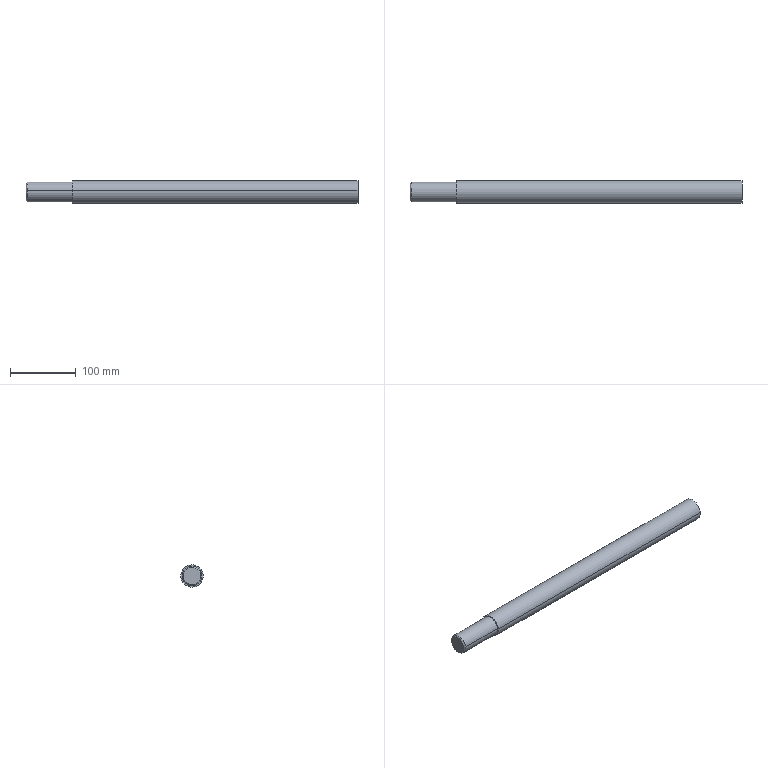Part | NX | features BREP 1 | 1 solid | 9 faces | box 504.795 x 33.982 x 33.982 mm | volume 443587 mm3 | cylinder 4 | plane 3 | cone 2 | commonest cylinder face diameters 30 x2 33.982 x2
STEP:
#1=CARTESIAN_POINT('',(560.635,-16.836,2.293));
#2=VERTEX_POINT('',#1);
#3=CARTESIAN_POINT('',(560.635,16.836,-2.293));
#4=VERTEX_POINT('',#3);
#5=CARTESIAN_POINT('',(560.635,0.,0.));
#6=DIRECTION('',(1.,0.,0.));
#7=DIRECTION('',(0.,0.,1.));
#8=AXIS2_PLACEMENT_3D('',#5,#6,#7);
#9=CIRCLE('',#8,16.991);
#10=EDGE_CURVE('',#2,#4,#9,.T.);
#11=ORIENTED_EDGE('',*,*,#10,.F.);
#12=CARTESIAN_POINT('',(126.35,-16.836,2.293));
#13=VERTEX_POINT('',#12);
#14=CARTESIAN_POINT('',(55.84,-16.836,2.293));
#15=DIRECTION('',(-1.,0.,0.));
#16=VECTOR('',#15,1000.);
#17=LINE('',#14,#16);
#18=EDGE_CURVE('',#2,#13,#17,.T.);
#19=ORIENTED_EDGE('',*,*,#18,.T.);
#20=CARTESIAN_POINT('',(126.35,16.836,-2.293));
#21=VERTEX_POINT('',#20);
#22=CARTESIAN_POINT('',(126.35,0.,0.));
#23=DIRECTION('',(1.,0.,0.));
#24=DIRECTION('',(0.,0.9909,-0.1349));
#25=AXIS2_PLACEMENT_3D('',#22,#23,#24);
#26=CIRCLE('',#25,16.991);
#27=EDGE_CURVE('',#13,#21,#26,.T.);
#28=ORIENTED_EDGE('',*,*,#27,.T.);
#29=CARTESIAN_POINT('',(55.84,16.836,-2.293));
#30=DIRECTION('',(-1.,0.,0.));
#31=VECTOR('',#30,1000.);
#32=LINE('',#29,#31);
#33=EDGE_CURVE('',#4,#21,#32,.T.);
#34=ORIENTED_EDGE('',*,*,#33,.F.);
#35=EDGE_LOOP('',(#11,#19,#28,#34));
#36=FACE_BOUND('',#35,.T.);
#37=CARTESIAN_POINT('',(55.84,0.,0.));
#38=DIRECTION('',(-1.,0.,0.));
#39=DIRECTION('',(0.,-0.9909,0.1349));
#40=AXIS2_PLACEMENT_3D('',#37,#38,#39);
#41=CYLINDRICAL_SURFACE('',#40,16.991);
#42=ADVANCED_FACE('',(#36),#41,.T.);
#43=CARTESIAN_POINT('',(126.35,14.863,-2.024));
#44=VERTEX_POINT('',#43);
#45=CARTESIAN_POINT('',(126.35,-14.863,2.024));
#46=VERTEX_POINT('',#45);
#47=CARTESIAN_POINT('',(126.35,0.,0.));
#48=DIRECTION('',(-1.,0.,0.));
#49=DIRECTION('',(0.,0.9909,-0.1349));
#50=AXIS2_PLACEMENT_3D('',#47,#48,#49);
#51=CIRCLE('',#50,15.);
#52=EDGE_CURVE('',#44,#46,#51,.T.);
#53=ORIENTED_EDGE('',*,*,#52,.T.);
#54=CARTESIAN_POINT('',(57.572,-14.863,2.024));
#55=VERTEX_POINT('',#54);
#56=CARTESIAN_POINT('',(55.84,-14.863,2.024));
#57=DIRECTION('',(-1.,0.,0.));
#58=VECTOR('',#57,1000.);
#59=LINE('',#56,#58);
#60=EDGE_CURVE('',#46,#55,#59,.T.);
#61=ORIENTED_EDGE('',*,*,#60,.T.);
#62=CARTESIAN_POINT('',(57.572,14.863,-2.024));
#63=VERTEX_POINT('',#62);
#64=CARTESIAN_POINT('',(57.572,0.,0.));
#65=DIRECTION('',(1.,0.,0.));
#66=DIRECTION('',(0.,0.9909,-0.1349));
#67=AXIS2_PLACEMENT_3D('',#64,#65,#66);
#68=CIRCLE('',#67,15.);
#69=EDGE_CURVE('',#55,#63,#68,.T.);
#70=ORIENTED_EDGE('',*,*,#69,.T.);
#71=CARTESIAN_POINT('',(55.84,14.863,-2.024));
#72=DIRECTION('',(-1.,0.,0.));
#73=VECTOR('',#72,1000.);
#74=LINE('',#71,#73);
#75=EDGE_CURVE('',#44,#63,#74,.T.);
#76=ORIENTED_EDGE('',*,*,#75,.F.);
#77=EDGE_LOOP('',(#53,#61,#70,#76));
#78=FACE_BOUND('',#77,.T.);
#79=CARTESIAN_POINT('',(55.84,0.,0.));
#80=DIRECTION('',(-1.,0.,0.));
#81=DIRECTION('',(0.,-0.9909,0.1349));
#82=AXIS2_PLACEMENT_3D('',#79,#80,#81);
#83=CYLINDRICAL_SURFACE('',#82,15.);
#84=ADVANCED_FACE('',(#78),#83,.T.);
#85=CARTESIAN_POINT('',(55.84,13.147,-1.79));
#86=VERTEX_POINT('',#85);
#87=CARTESIAN_POINT('',(55.84,-13.147,1.79));
#88=VERTEX_POINT('',#87);
#89=CARTESIAN_POINT('',(55.84,0.,0.));
#90=DIRECTION('',(-1.,0.,0.));
#91=DIRECTION('',(0.,0.9909,-0.1349));
#92=AXIS2_PLACEMENT_3D('',#89,#90,#91);
#93=CIRCLE('',#92,13.268);
#94=EDGE_CURVE('',#86,#88,#93,.T.);
#95=ORIENTED_EDGE('',*,*,#94,.F.);
#96=CARTESIAN_POINT('',(55.84,13.147,-1.79));
#97=DIRECTION('',(0.7071,0.7006,-0.09541));
#98=VECTOR('',#97,1000.);
#99=LINE('',#96,#98);
#100=EDGE_CURVE('',#63,#86,#99,.F.);
#101=ORIENTED_EDGE('',*,*,#100,.F.);
#102=ORIENTED_EDGE('',*,*,#69,.F.);
#103=CARTESIAN_POINT('',(55.84,-13.147,1.79));
#104=DIRECTION('',(0.7071,-0.7006,0.09541));
#105=VECTOR('',#104,1000.);
#106=LINE('',#103,#105);
#107=EDGE_CURVE('',#55,#88,#106,.F.);
#108=ORIENTED_EDGE('',*,*,#107,.T.);
#109=EDGE_LOOP('',(#95,#101,#102,#108));
#110=FACE_BOUND('',#109,.T.);
#111=CARTESIAN_POINT('',(55.84,0.,0.));
#112=DIRECTION('',(1.,0.,0.));
#113=DIRECTION('',(0.,0.9909,-0.1349));
#114=AXIS2_PLACEMENT_3D('',#111,#112,#113);
#115=CONICAL_SURFACE('',#114,13.268,0.7854);
#116=ADVANCED_FACE('',(#110),#115,.T.);
#117=CARTESIAN_POINT('',(55.84,0.,0.));
#118=DIRECTION('',(-1.,0.,0.));
#119=DIRECTION('',(0.,0.9909,-0.1349));
#120=AXIS2_PLACEMENT_3D('',#117,#118,#119);
#121=CIRCLE('',#120,13.268);
#122=EDGE_CURVE('',#88,#86,#121,.T.);
#123=ORIENTED_EDGE('',*,*,#122,.T.);
#124=ORIENTED_EDGE('',*,*,#94,.T.);
#125=EDGE_LOOP('',(#123,#124));
#126=FACE_BOUND('',#125,.T.);
#127=CARTESIAN_POINT('',(55.84,14.863,-2.024));
#128=DIRECTION('',(-1.,0.,0.));
#129=DIRECTION('',(0.,-0.9909,0.1349));
#130=AXIS2_PLACEMENT_3D('',#127,#128,#129);
#131=PLANE('',#130);
#132=ADVANCED_FACE('',(#126),#131,.T.);
#133=ORIENTED_EDGE('',*,*,#100,.T.);
#134=ORIENTED_EDGE('',*,*,#122,.F.);
#135=ORIENTED_EDGE('',*,*,#107,.F.);
#136=CARTESIAN_POINT('',(57.572,0.,0.));
#137=DIRECTION('',(1.,0.,0.));
#138=DIRECTION('',(0.,0.9909,-0.1349));
#139=AXIS2_PLACEMENT_3D('',#136,#137,#138);
#140=CIRCLE('',#139,15.);
#141=EDGE_CURVE('',#63,#55,#140,.T.);
#142=ORIENTED_EDGE('',*,*,#141,.F.);
#143=EDGE_LOOP('',(#133,#134,#135,#142));
#144=FACE_BOUND('',#143,.T.);
#145=CARTESIAN_POINT('',(55.84,0.,0.));
#146=DIRECTION('',(1.,0.,0.));
#147=DIRECTION('',(0.,0.9909,-0.1349));
#148=AXIS2_PLACEMENT_3D('',#145,#146,#147);
#149=CONICAL_SURFACE('',#148,13.268,0.7854);
#150=ADVANCED_FACE('',(#144),#149,.T.);
#151=ORIENTED_EDGE('',*,*,#60,.F.);
#152=CARTESIAN_POINT('',(126.35,0.,0.));
#153=DIRECTION('',(-1.,0.,0.));
#154=DIRECTION('',(0.,0.9909,-0.1349));
#155=AXIS2_PLACEMENT_3D('',#152,#153,#154);
#156=CIRCLE('',#155,15.);
#157=EDGE_CURVE('',#46,#44,#156,.T.);
#158=ORIENTED_EDGE('',*,*,#157,.T.);
#159=ORIENTED_EDGE('',*,*,#75,.T.);
#160=ORIENTED_EDGE('',*,*,#141,.T.);
#161=EDGE_LOOP('',(#151,#158,#159,#160));
#162=FACE_BOUND('',#161,.T.);
#163=CARTESIAN_POINT('',(55.84,0.,0.));
#164=DIRECTION('',(-1.,0.,0.));
#165=DIRECTION('',(0.,-0.9909,0.1349));
#166=AXIS2_PLACEMENT_3D('',#163,#164,#165);
#167=CYLINDRICAL_SURFACE('',#166,15.);
#168=ADVANCED_FACE('',(#162),#167,.T.);
#169=CARTESIAN_POINT('',(126.35,0.,0.));
#170=DIRECTION('',(1.,0.,0.));
#171=DIRECTION('',(0.,0.9909,-0.1349));
#172=AXIS2_PLACEMENT_3D('',#169,#170,#171);
#173=CIRCLE('',#172,16.991);
#174=EDGE_CURVE('',#21,#13,#173,.T.);
#175=ORIENTED_EDGE('',*,*,#174,.F.);
#176=ORIENTED_EDGE('',*,*,#27,.F.);
#177=EDGE_LOOP('',(#175,#176));
#178=FACE_BOUND('',#177,.T.);
#179=ORIENTED_EDGE('',*,*,#52,.F.);
#180=ORIENTED_EDGE('',*,*,#157,.F.);
#181=EDGE_LOOP('',(#179,#180));
#182=FACE_BOUND('',#181,.T.);
#183=CARTESIAN_POINT('',(126.35,16.836,-2.293));
#184=DIRECTION('',(-1.,0.,0.));
#185=DIRECTION('',(0.,-0.9909,0.1349));
#186=AXIS2_PLACEMENT_3D('',#183,#184,#185);
#187=PLANE('',#186);
#188=ADVANCED_FACE('',(#178,#182),#187,.T.);
#189=ORIENTED_EDGE('',*,*,#18,.F.);
#190=CARTESIAN_POINT('',(560.635,0.,0.));
#191=DIRECTION('',(1.,0.,0.));
#192=DIRECTION('',(0.,0.,1.));
#193=AXIS2_PLACEMENT_3D('',#190,#191,#192);
#194=CIRCLE('',#193,16.991);
#195=EDGE_CURVE('',#4,#2,#194,.T.);
#196=ORIENTED_EDGE('',*,*,#195,.F.);
#197=ORIENTED_EDGE('',*,*,#33,.T.);
#198=ORIENTED_EDGE('',*,*,#174,.T.);
#199=EDGE_LOOP('',(#189,#196,#197,#198));
#200=FACE_BOUND('',#199,.T.);
#201=CARTESIAN_POINT('',(55.84,0.,0.));
#202=DIRECTION('',(-1.,0.,0.));
#203=DIRECTION('',(0.,-0.9909,0.1349));
#204=AXIS2_PLACEMENT_3D('',#201,#202,#203);
#205=CYLINDRICAL_SURFACE('',#204,16.991);
#206=ADVANCED_FACE('',(#200),#205,.T.);
#207=ORIENTED_EDGE('',*,*,#195,.T.);
#208=ORIENTED_EDGE('',*,*,#10,.T.);
#209=EDGE_LOOP('',(#207,#208));
#210=FACE_BOUND('',#209,.T.);
#211=CARTESIAN_POINT('',(560.635,0.,0.));
#212=DIRECTION('',(-1.,0.,0.));
#213=DIRECTION('',(0.,0.,-1.));
#214=AXIS2_PLACEMENT_3D('',#211,#212,#213);
#215=PLANE('',#214);
#216=ADVANCED_FACE('',(#210),#215,.F.);
#217=CLOSED_SHELL('',(#42,#84,#116,#132,#150,#168,#188,#206,#216));
#218=MANIFOLD_SOLID_BREP('',#217);
#219=(LENGTH_UNIT()NAMED_UNIT(*)SI_UNIT(.MILLI.,.METRE.));
#220=UNCERTAINTY_MEASURE_WITH_UNIT(LENGTH_MEASURE(0.00001),#219,'','');
#221=(NAMED_UNIT(*)PLANE_ANGLE_UNIT()SI_UNIT($,.RADIAN.));
#222=(NAMED_UNIT(*)SI_UNIT($,.STERADIAN.)SOLID_ANGLE_UNIT());
#223=(GEOMETRIC_REPRESENTATION_CONTEXT(3)GLOBAL_UNCERTAINTY_ASSIGNED_CONTEXT((#220))GLOBAL_UNIT_ASSIGNED_CONTEXT((#219,#221,#222))REPRESENTATION_CONTEXT('',''));
#224=ADVANCED_BREP_SHAPE_REPRESENTATION('',(#218),#223);